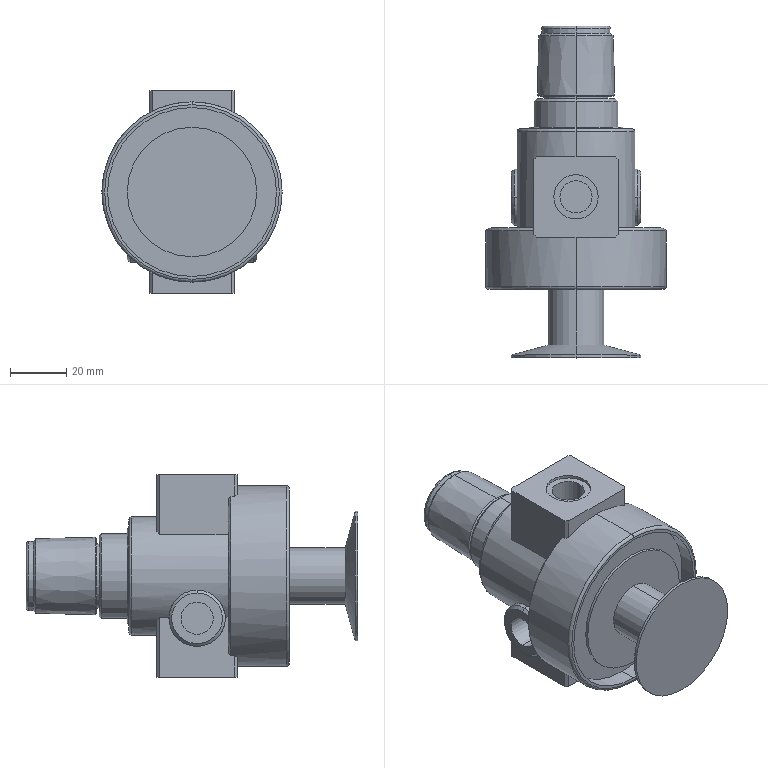Part | SolidWorks | features BaseBody 1 | 1 solid | 99 faces | box 64 x 117.8 x 72 mm | volume 166401 mm3 | plane 37 | cylinder 36 | cone 20 | torus 6 | commonest cylinder face diameters 11.445 x8 20 x8 15.788 x4 46 x4 23 x2 24.545 x2